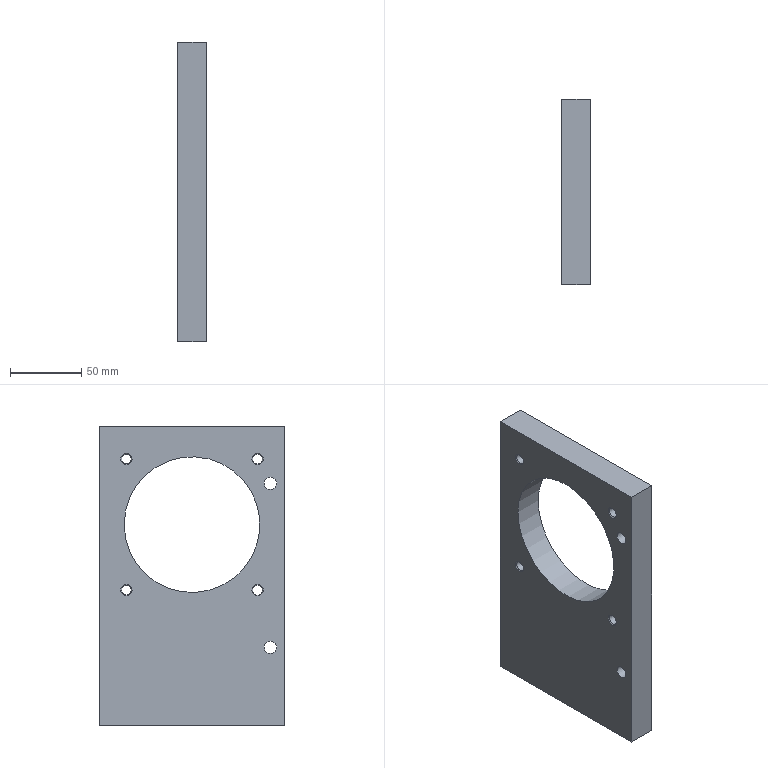Part | STEP file | YBQDJ-YB-21 | 1 solid | 31 faces | box 20 x 130 x 210 mm | volume 393461 mm3 | cone 12 | cylinder 11 | plane 8 | commonest cylinder face diameters 6.8 x4 8.5 x2 8.7 x2 14 x2 95.1 x1